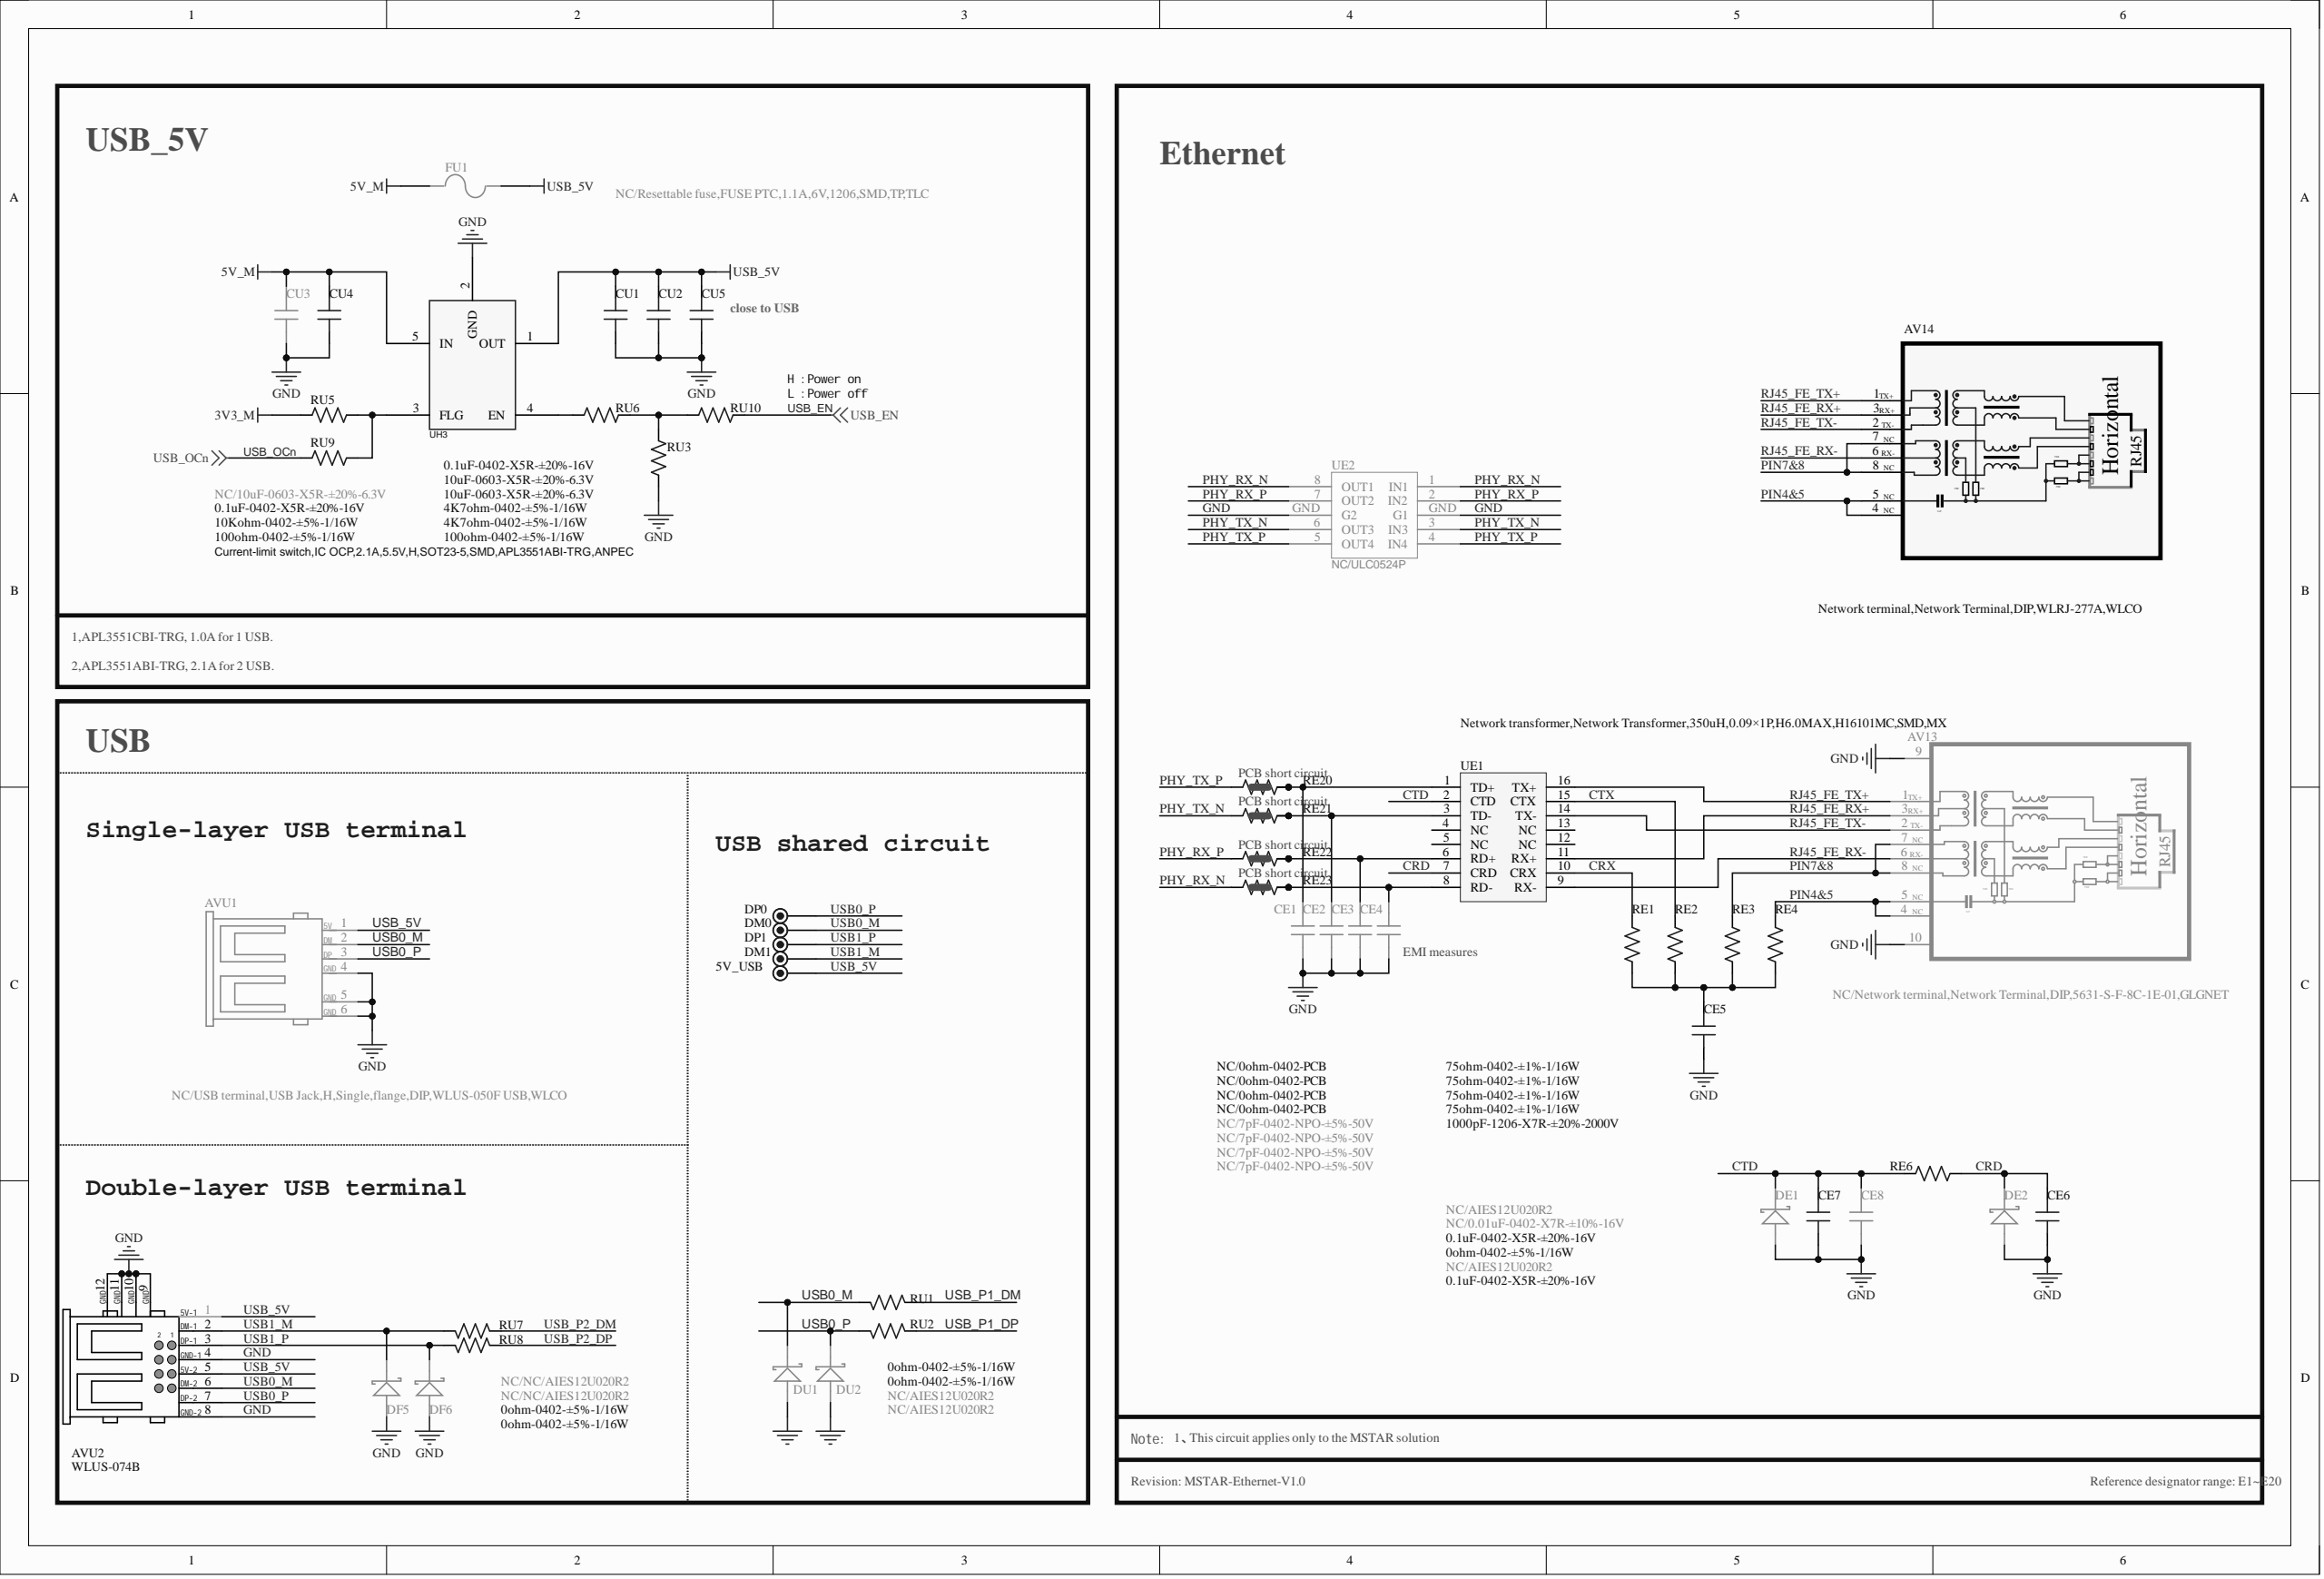Circuit board | Altium Designer | 1029 parts | 642 nets | one sheet of the schematic
Parts on this sheet (reference | value | footprint):
5V_USB | TEST | TP
AV13 | NC/Network terminal,Network Terminal,DIP,5631-S-F-8C-1E-01,GLGNET | RJ45U-D-5
AV14 | Network terminal,Network Terminal,DIP,WLRJ-277A,WLCO | RJ45U-D-14
AVU1 | NC/USB terminal,USB Jack,H,Single,flange,DIP,WLUS-050F USB,WLCO | USB1-HD-2
AVU2 | WLUS-074B | USB2-HD-1
CE1 | NC/7pF-0402-NPO-±5%-50V | C0402
CE2 | NC/7pF-0402-NPO-±5%-50V | C0402
CE3 | NC/7pF-0402-NPO-±5%-50V | C0402
CE4 | NC/7pF-0402-NPO-±5%-50V | C0402
CE5 | 1000pF-1206-X7R-±20%-2000V | C1206
CE6 | 0.1uF-0402-X5R-±20%-16V | C0402
CE7 | 0.1uF-0402-X5R-±20%-16V | C0402
CE8 | NC/0.01uF-0402-X7R-±10%-16V | C0402
CU1 | 0.1uF-0402-X5R-±20%-16V | C0402
CU2 | 10uF-0603-X5R-±20%-6.3V | C0603
CU3 | NC/10uF-0603-X5R-±20%-6.3V | C0603
CU4 | 0.1uF-0402-X5R-±20%-16V | C0402
CU5 | 10uF-0603-X5R-±20%-6.3V | C0603
DE1 | NC/AIES12U020R2 | DIODE-S0402
DE2 | NC/AIES12U020R2 | DIODE-S0402
DF5 | NC/NC/AIES12U020R2 | DIODE-S0402
DF6 | NC/NC/AIES12U020R2 | DIODE-S0402
DM0 | TEST | TP
DM1 | TEST | TP
DP0 | TEST | TP
DP1 | TEST | TP
DU1 | NC/AIES12U020R2 | DIODE-S0402
DU2 | NC/AIES12U020R2 | DIODE-S0402
FU1 | NC/Resettable fuse,FUSE PTC,1.1A,6V,1206,SMD,TP,TLC | FUSE1.1A-S
RE1 | 75ohm-0402-±1%-1/16W | R0402
RE2 | 75ohm-0402-±1%-1/16W | R0402
RE3 | 75ohm-0402-±1%-1/16W | R0402
RE4 | 75ohm-0402-±1%-1/16W | R0402
RE6 | 0ohm-0402-±5%-1/16W | R0402
RE20 | NC/0ohm-0402-PCB | R0402SC
RE21 | NC/0ohm-0402-PCB | R0402SC
RE22 | NC/0ohm-0402-PCB | R0402SC
RE23 | NC/0ohm-0402-PCB | R0402SC
RU1 | 0ohm-0402-±5%-1/16W | R0402
RU2 | 0ohm-0402-±5%-1/16W | R0402
RU3 | 4K7ohm-0402-±5%-1/16W | R0402
RU5 | 10Kohm-0402-±5%-1/16W | R0402
RU6 | 4K7ohm-0402-±5%-1/16W | R0402
RU7 | 0ohm-0402-±5%-1/16W | R0402
RU8 | 0ohm-0402-±5%-1/16W | R0402
RU9 | 100ohm-0402-±5%-1/16W | R0402
RU10 | 100ohm-0402-±5%-1/16W | R0402
UE1 | Network transformer,Network Transformer,350uH,0.09×1P,H6.0MAX,H16101MC,SMD,MX | SOP16/1.27-2
UE2 | NC/ULC0524P | RCL0524P
UH3 | Current-limit switch,IC OCP,2.1A,5.5V,H,SOT23-5,SMD,APL3551ABI-TRG,ANPEC | SOT-23-5
Nets of these parts (net: part-pin ...):
USB_P2_DP: RU8-1
USB_P2_DM: RU7-1
USB_P1_DP: RU2-1
USB_P1_DM: RU1-1
USB_OCn: RU9-1
USB_EN: RU10-2
USB_5V: 5V_USB-1 AVU1-1 AVU2-1 AVU2-5 CU1-1 CU2-1 CU5-1 FU1-2 UH3-1
USB1_P: AVU2-3 DF6-K DP1-1 RU8-2
USB1_M: AVU2-2 DF5-K DM1-1 RU7-2
USB0_P: AVU1-3 AVU2-7 DP0-1 DU2-K RU2-2
USB0_M: AVU1-2 AVU2-6 DM0-1 DU1-K RU1-2
RJ45_FE_TX-: AV13-2 AV14-2 UE1-14
RJ45_FE_TX+: AV13-1 AV14-1 UE1-16
RJ45_FE_RX-: AV13-6 AV14-6 UE1-9
RJ45_FE_RX+: AV13-3 AV14-3 UE1-11
PIN7&8: AV13-7 AV13-8 AV14-7 AV14-8 RE3-2
PIN4&5: AV13-4 AV13-5 AV14-4 AV14-5 RE4-2
PHY_TX_P: RE20-1 UE2-4 UE2-5
PHY_TX_N: RE21-1 UE2-3 UE2-6
PHY_RX_P: RE22-1 UE2-2 UE2-7
PHY_RX_N: RE23-1 UE2-1 UE2-8
NetRU6_2: RU6-2 UH3-4
NetRU5_2: RU5-2 RU9-2 UH3-3
NetRU3_1: RU3-1 RU6-1 RU10-1
NetCE5_1: CE5-1 RE1-1 RE2-1 RE3-1 RE4-1
NetCE4_2: CE4-2 RE23-2 RE23-3 UE1-8
NetCE3_2: CE3-2 RE22-2 RE22-3 UE1-6
NetCE2_2: CE2-2 RE21-2 RE21-3 UE1-3
NetCE1_2: CE1-2 RE20-2 RE20-3 UE1-1
GND: AV13-9 AV13-10 AVU1-4 AVU1-5 AVU1-6 AVU2-4 AVU2-8 AVU2-9 AVU2-10 AVU2-11 AVU2-12 CE1-1 CE2-1 CE3-1 CE4-1 CE5-2 CE6-2 CE7-1 CE8-1 CU1-2 CU2-2 CU3-1 CU4-1 CU5-2 DE1-A DE2-A DF5-A DF6-A DU1-A DU2-A RU3-2 UE2-GND UH3-2
CTX: RE2-2 UE1-15
CTD: CE7-2 CE8-2 DE1-K RE6-1 UE1-2
CRX: RE1-2 UE1-10
CRD: CE6-1 DE2-K RE6-2 UE1-7
5V_M: CU3-2 CU4-2 FU1-1 UH3-5
3V3_M: RU5-1